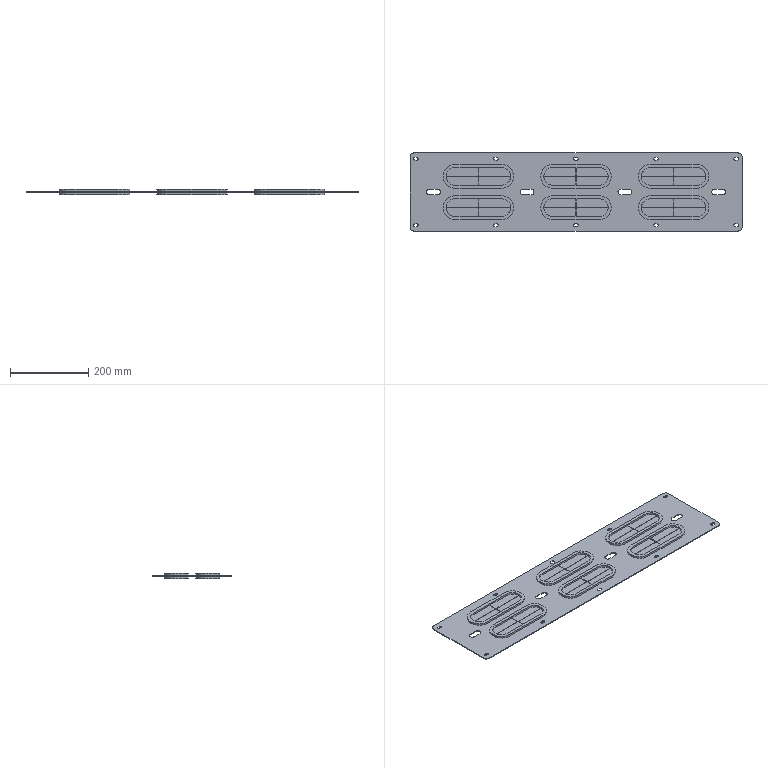Part | SolidWorks | 7 solids | 434 faces | box 850 x 200 x 14 mm | volume 624730 mm3 | plane 310 | cylinder 124 | commonest cylinder face diameters 7 x30 50 x30 45 x24 61 x24 15 x12 20 x4